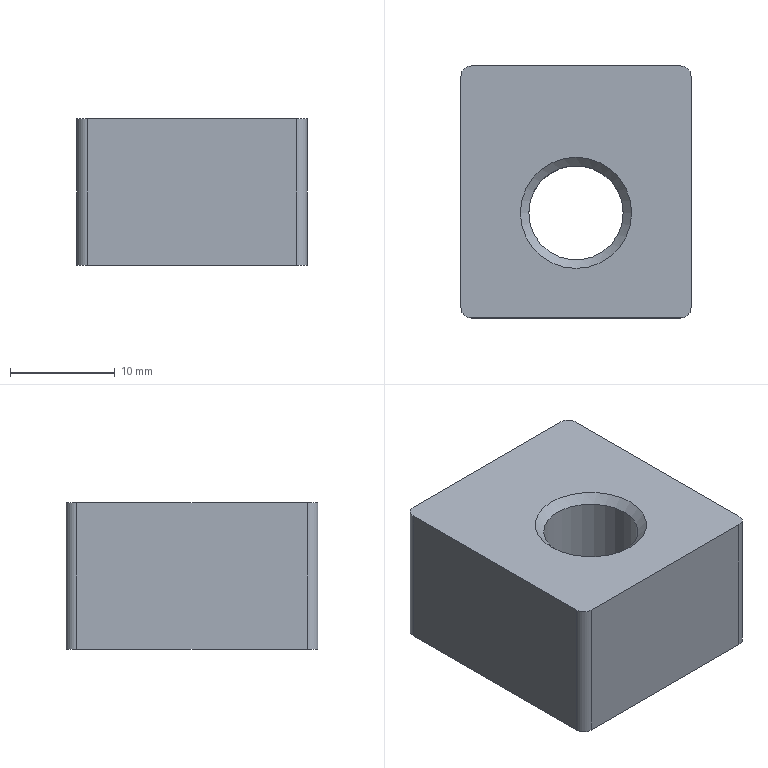NC program | NX | posted with a generic post | part box 21.95 x 24 x 14 mm
Whole program:
N10 G17 G21 G94 G90
(ADAPTIVE_MILLING , TOOL : D16CU)
N12 T01 M6
N14 G53
N16 G17 G0 G90 X-12.052 Y27.556 S2800 M3
N18 G43 Z50.1 H1
N20 Z-12.
N22 G94 G1 X-12.059 Y27.406 Z-12.937 F3000.
N24 X-12.066 Y27.256 Z-13.308
N26 X-12.072 Y27.106 Z-13.58
N28 X-12.079 Y26.956 Z-13.8
N30 X-12.086 Y26.807 Z-13.984
N32 X-12.093 Y26.657 Z-14.142
N34 X-12.099 Y26.507 Z-14.28
N36 X-12.106 Y26.357 Z-14.4
N38 X-12.113 Y26.207 Z-14.505
N40 X-12.12 Y26.057 Z-14.598
N42 X-12.127 Y25.907 Z-14.679
N44 X-12.133 Y25.758 Z-14.75
N46 X-12.14 Y25.608 Z-14.81
N48 X-12.147 Y25.458 Z-14.862
N50 X-12.154 Y25.308 Z-14.905
N52 X-12.16 Y25.158 Z-14.939
N54 X-12.167 Y25.008 Z-14.966
N56 X-12.174 Y24.859 Z-14.985
N58 X-12.181 Y24.709 Z-14.996
N60 X-12.188 Y24.559 Z-15.
N62 X-12.296 Y22.159
N64 G3 X-11.107 Y20.527 R1.616
N66 X-7.999 Y20.23 R16.908
N68 X4.363 Y20.148 R484.421
N70 G2 X11.712 Y20.13 R529.449
N72 X17.987 Y16.718 R8.91
N74 X20.544 Y10.933 R13.171
N76 X21.096 Y4.621 R36.918
N78 X21.136 Y-10.641 R809.045
N80 X17.768 Y-16.939 R8.895
N82 X12.039 Y-19.519 R13.086
N84 X5.73 Y-20.092 R35.808
N86 X-11.617 Y-20.138 R898.541
N88 X-17.926 Y-16.791 R8.882
N90 X-20.524 Y-11.023 R13.079
N92 X-21.092 Y-4.757 R35.849
N94 X-21.132 Y10.704 R800.369
N96 X-17.179 Y17.372 R8.922
N98 X-11.566 Y19.446 R13.178
N100 X-5.63 Y19.787 R43.63
N102 X9.527 Y19.78 R971.623
N104 X13.764 Y18.642 R10.666
N106 G1 X15.132 Y18.083
N108 X16.35 Y17.336
N110 X17.435 Y16.409
N112 X18.363 Y15.323
N114 X19.109 Y14.105
N116 X19.709 Y12.62
N118 G2 X20.669 Y5.185 R36.65
N120 X20.781 Y-8.507 R327.819
N122 X19.674 Y-12.709 R11.291
N124 G1 X19.108 Y-14.107
N126 X18.361 Y-15.325
N128 X17.434 Y-16.41
N130 X16.348 Y-17.338
N132 X15.13 Y-18.084
N134 X13.645 Y-18.684
N136 G2 X5.717 Y-19.685 R37.838
N138 X-9.551 Y-19.78 R422.895
N140 X-13.789 Y-18.635 R11.097
N142 G1 X-15.132 Y-18.083
N144 X-16.35 Y-17.336
N146 X-17.435 Y-16.409
N148 X-18.363 Y-15.323
N150 X-19.109 Y-14.105
N152 X-19.709 Y-12.62
N154 G2 X-20.666 Y-5.228 R36.564
N156 X-20.776 Y8.595 R317.687
N158 X-19.698 Y12.626 R10.569
N160 X-19.108 Y14.107 R15.265
N162 G1 X-18.361 Y15.325
N164 X-17.434 Y16.41
N166 X-16.348 Y17.338
N168 X-15.13 Y18.084
N170 X-13.811 Y18.63
N172 G2 X-10.379 Y19.185 R15.543
N174 X-2.072 Y19.439 R108.841
N176 X7.789 Y19.425 R597.03
N178 X10.476 Y19.075 R25.298
N180 X12.425 Y18.963 R16.48
N182 G1 X13.813 Y18.629
N184 X15.132 Y18.083
N186 X16.35 Y17.336
N188 X17.435 Y16.409
N190 X18.363 Y15.323
N192 X19.109 Y14.105
N194 X19.655 Y12.786
N196 X19.988 Y11.397
N198 G2 X20.307 Y5.161 R141.056
N200 X20.421 Y-6.825 R270.037
N202 X20.1 Y-9.341 R23.433
N204 X19.988 Y-11.4 R16.151
N206 G1 X19.661 Y-12.761
N208 G3 X22.062 Y-14.493 R1.6
N210 X22.638 Y-13.886 Z-14.974 R1.792
N212 G1 X23.929 Y-11.931 Z-14.9
N214 X24.832 Y-10.564 F15000.
N216 G3 X25.096 Y-9.623 R1.605
N218 G1 X24.538 Y5.537
N220 X24.518 Y5.721
N222 X24.481 Y5.903
N224 X24.088 Y7.329
N226 X23.242 Y10.402 Z-15. F3000.
N228 G3 X20.1 Y9.974 R1.6
N230 G1 Y-9.976
N232 X19.988 Y-11.4
N234 X19.654 Y-12.788
N236 X19.108 Y-14.107
N238 X18.361 Y-15.325
N240 X17.434 Y-16.41
N242 X16.348 Y-17.338
N244 X15.13 Y-18.084
N246 X13.811 Y-18.63
N248 X12.422 Y-18.963
N250 G2 X-0.89 Y-19.432 R175.68
N252 X-7.933 Y-19.418 R217.752
N254 X-10.489 Y-19.075 R29.81
N256 X-12.425 Y-18.963 R16.571
N258 G1 X-13.813 Y-18.629
N260 G3 X-15.539 Y-21.041 R1.6
N262 X-14.936 Y-21.607 Z-14.974 R1.796
N264 G1 X-12.971 Y-22.902 Z-14.9
N266 X-11.607 Y-23.801 F15000.
N268 G3 X-10.675 Y-24.064 R1.605
N270 G1 X6.562 Y-23.513
N272 X6.75 Y-23.493
N274 X6.936 Y-23.456
N276 X8.358 Y-23.063
N278 X11.431 Y-22.216 Z-15. F3000.
N280 G3 X10.999 Y-19.075 R1.6
N282 G1 X-11.001
N284 X-12.425 Y-18.963
N286 X-13.813 Y-18.629
N288 X-15.132 Y-18.083
N290 X-16.35 Y-17.336
N292 X-17.435 Y-16.409
N294 X-18.363 Y-15.323
N296 X-19.109 Y-14.105
N298 X-19.655 Y-12.786
N300 X-19.988 Y-11.397
N302 G2 X-20.306 Y-5.154 R140.928
N304 X-20.422 Y6.788 R283.557
N306 X-20.1 Y9.341 R27.12
N308 X-19.988 Y11.4 R16.151
N310 G1 X-19.671 Y12.718
N312 G3 X-22.061 Y14.457 R1.6
N314 X-22.647 Y13.844 Z-14.973 R1.787
N316 G1 X-23.932 Y11.899 Z-14.9
N318 X-24.842 Y10.523 F15000.
N320 G3 X-25.106 Y9.581 R1.605
N322 G1 X-24.538 Y-5.537
N324 X-24.518 Y-5.721
N326 X-24.481 Y-5.902
N328 X-24.088 Y-7.328
N330 X-23.242 Y-10.401 Z-15. F3000.
N332 G3 X-20.1 Y-9.974 R1.6
N334 G1 Y9.976
N336 X-19.988 Y11.4
N338 X-19.654 Y12.788
N340 X-19.108 Y14.107
N342 X-18.361 Y15.325
N344 X-17.434 Y16.41
N346 X-16.348 Y17.338
N348 X-15.13 Y18.084
N350 X-13.811 Y18.63
N352 X-12.422 Y18.963
N354 X-10.999 Y19.075
N356 X10.482
N358 G3 X12.042 Y20.27 R1.616
N360 G1 X12.761 Y22.932
N362 X12.8 Y23.077 Z-14.996
N364 X12.839 Y23.222 Z-14.985
N366 X12.878 Y23.367 Z-14.966
N368 X12.917 Y23.511 Z-14.939
N370 X12.956 Y23.656 Z-14.905
N372 X12.996 Y23.801 Z-14.862
N374 X13.035 Y23.946 Z-14.81
N376 X13.074 Y24.091 Z-14.75
N378 X13.113 Y24.235 Z-14.679
N380 X13.152 Y24.38 Z-14.598
N382 X13.191 Y24.525 Z-14.505
N384 X13.23 Y24.67 Z-14.4
N386 X13.269 Y24.815 Z-14.28
N388 X13.308 Y24.96 Z-14.142
N390 X13.347 Y25.104 Z-13.984
N392 X13.387 Y25.249 Z-13.8
N394 X13.426 Y25.394 Z-13.58
N396 X13.465 Y25.539 Z-13.308
N398 X13.504 Y25.684 Z-12.937
N400 X13.543 Y25.828 Z-12.
N402 G0 Z50.1
(PLANAR_MILL_COPY_1_COPY , TOOL : D16CU)
N404 X-4. Y20.201 S2500
N406 Z50.
N408 Z0.
N410 G1 Y12.3 F400.
N412 G3 X-2. Y10.3 R2.
N414 G2 X8.3 Y0. R10.3
N416 X-2. Y10.3 R-10.3
N418 G3 X0. Y12.3 R2.
N420 G1 Y20.201
N422 G0 Z50.
N424 M5
(PLANAR_MILL , TOOL : D16.)
N426 T02 M6
N428 G53
N430 G17 G0 G90 X9. Y21.025 S1600 M3
N432 G43 Z50. H2
N434 Z-14.3
N436 G94 G3 X11. Y19.025 R2. F400.
N438 G2 X20.05 Y9.975 R9.05
N440 G1 Y-9.975
N442 G2 X11. Y-19.025 R9.05
N444 G1 X-11.
N446 G2 X-20.05 Y-9.975 R9.05
N448 G1 Y9.975
N450 G2 X-11. Y19.025 R9.05
N452 G1 X11.
N454 G3 X12.992 Y20.844 R2.
N456 G1 X9. Y20.975
N458 G3 X11. Y18.975 R2.
N460 G2 X20. Y9.975 R9.
N462 G1 Y-9.975
N464 G2 X11. Y-18.975 R9.
N466 G1 X-11.
N468 G2 X-20. Y-9.975 R9.
N470 G1 Y9.975
N472 G2 X-11. Y18.975 R9.
N474 G1 X11.
N476 G3 X12.996 Y20.843 R2.
N478 G0 Z50.
(PLANAR_MILL_COPY_1 , TOOL : D16.)
N480 Z50.
N482 X-4. Y20.704
N484 Z0.
N486 G1 Y12.8
N488 G3 X-2. Y10.8 R2.
N490 G2 X8.8 Y0. R10.8
N492 X-2. Y10.8 R-10.8
N494 G3 X0. Y12.8 R2.
N496 G1 Y20.704
N498 G0 Z50.
N500 M5
(PLANAR_MILL_COPY , TOOL : D8点钻)
N502 T03 M6
N504 G53
N506 G17 G0 G90 X-16.8 Y7.975 S4500 M3
N508 G43 Z50. H3
N510 Z-3.
N512 G94 G3 X-14.8 Y9.975 R2. F1200.
N514 G2 X-11. Y13.775 R3.8
N516 G1 X11.
N518 G2 X14.8 Y9.975 R3.8
N520 G1 Y-9.975
N522 G2 X11. Y-13.775 R3.8
N524 G1 X-11.
N526 G2 X-14.8 Y-9.975 R3.8
N528 G1 Y9.975
N530 G3 X-16.455 Y11.945 R2.
N532 G0 Z50.
(PLANAR_MILL_COPY_COPY_COPY_COPY , TOOL : D8点钻)
N534 X-1. Y0.831
N536 Z-3.
N538 G1 Y1.3
N540 G3 X-2. Y2.3 R1.
N542 X-4.3 Y0. R2.3
N544 X-2. Y2.3 R-2.3
N546 X-3. Y1.3 R1.
N548 G1 Y0.831
N550 G0 Z50.
(DRILLING , TOOL : D8点钻)
N552 X-2. Y0. S0
N554 Z20.
N556 G81 G98 Z0. F250. R3.
N558 G80
N560 G0 X-2. Y0. Z20.
N562 M5
(DRILLING_COPY , TOOL : Z9.)
N564 T09 M6
N566 G53
N568 G17 G0 G90 X-2. Y0. S800 M3
N570 G43 Z20. H9
N572 G94 G83 G98 Z-22. F100. Q2. R3.
N574 G80
N576 G0 X-2. Y0. Z20.
N578 M5
N580 M2